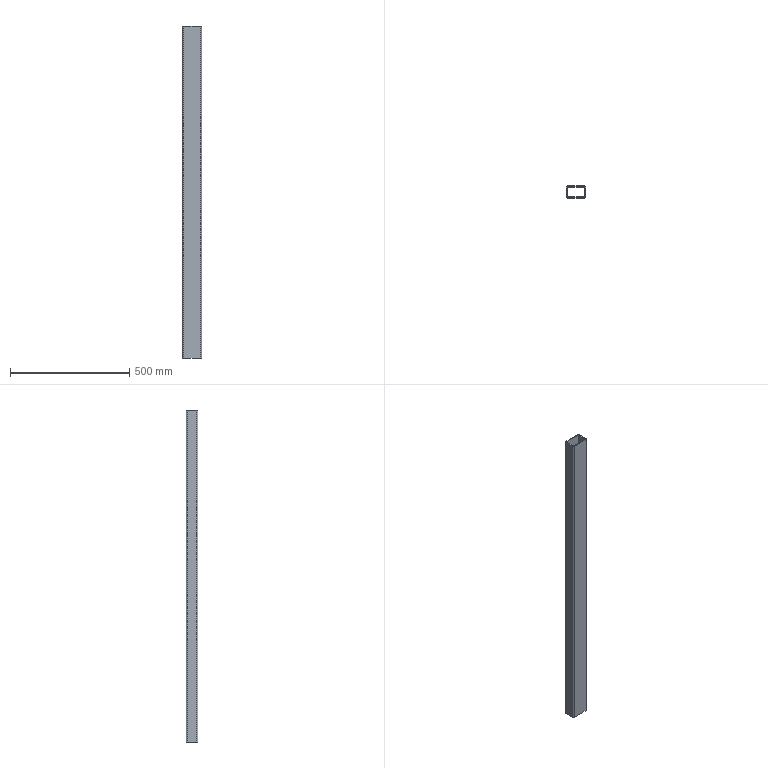Part | SolidWorks | features Extrusion 1, Shell 1 | 1 solid | 18 faces | box 80 x 50 x 1393 mm | volume 1330870 mm3 | plane 10 | cylinder 8 | commonest cylinder face diameters 2 x4 10 x4
STEP:
#1=CARTESIAN_POINT('',(-35.,25.,0.));
#2=VERTEX_POINT('',#1);
#3=CARTESIAN_POINT('',(-40.,20.,0.));
#4=VERTEX_POINT('',#3);
#5=CARTESIAN_POINT('',(-35.,20.,0.));
#6=DIRECTION('',(0.,0.,1.));
#7=DIRECTION('',(1.,0.,0.));
#8=AXIS2_PLACEMENT_3D('',#5,#6,#7);
#9=CIRCLE('',#8,5.);
#10=EDGE_CURVE('',#2,#4,#9,.T.);
#11=ORIENTED_EDGE('',*,*,#10,.T.);
#12=CARTESIAN_POINT('',(-40.,20.,1393.));
#13=VERTEX_POINT('',#12);
#14=CARTESIAN_POINT('',(-40.,20.,1393.));
#15=DIRECTION('',(0.,0.,-1.));
#16=VECTOR('',#15,1000.);
#17=LINE('',#14,#16);
#18=EDGE_CURVE('',#13,#4,#17,.T.);
#19=ORIENTED_EDGE('',*,*,#18,.F.);
#20=CARTESIAN_POINT('',(-35.,25.,1393.));
#21=VERTEX_POINT('',#20);
#22=CARTESIAN_POINT('',(-35.,20.,1393.));
#23=DIRECTION('',(0.,0.,1.));
#24=DIRECTION('',(1.,0.,0.));
#25=AXIS2_PLACEMENT_3D('',#22,#23,#24);
#26=CIRCLE('',#25,5.);
#27=EDGE_CURVE('',#21,#13,#26,.T.);
#28=ORIENTED_EDGE('',*,*,#27,.F.);
#29=CARTESIAN_POINT('',(-35.,25.,1393.));
#30=DIRECTION('',(0.,0.,-1.));
#31=VECTOR('',#30,1000.);
#32=LINE('',#29,#31);
#33=EDGE_CURVE('',#21,#2,#32,.T.);
#34=ORIENTED_EDGE('',*,*,#33,.T.);
#35=EDGE_LOOP('',(#11,#19,#28,#34));
#36=FACE_OUTER_BOUND('',#35,.T.);
#37=CARTESIAN_POINT('',(-35.,20.,1393.));
#38=DIRECTION('',(0.,0.,-1.));
#39=DIRECTION('',(-1.,0.,0.));
#40=AXIS2_PLACEMENT_3D('',#37,#38,#39);
#41=CYLINDRICAL_SURFACE('',#40,5.);
#42=ADVANCED_FACE('',(#36),#41,.T.);
#43=CARTESIAN_POINT('',(-40.,-20.,0.));
#44=VERTEX_POINT('',#43);
#45=CARTESIAN_POINT('',(-40.,20.,0.));
#46=DIRECTION('',(0.,-1.,0.));
#47=VECTOR('',#46,1000.);
#48=LINE('',#45,#47);
#49=EDGE_CURVE('',#4,#44,#48,.T.);
#50=ORIENTED_EDGE('',*,*,#49,.T.);
#51=CARTESIAN_POINT('',(-40.,-20.,1393.));
#52=VERTEX_POINT('',#51);
#53=CARTESIAN_POINT('',(-40.,-20.,1393.));
#54=DIRECTION('',(0.,0.,-1.));
#55=VECTOR('',#54,1000.);
#56=LINE('',#53,#55);
#57=EDGE_CURVE('',#52,#44,#56,.T.);
#58=ORIENTED_EDGE('',*,*,#57,.F.);
#59=CARTESIAN_POINT('',(-40.,20.,1393.));
#60=DIRECTION('',(0.,-1.,0.));
#61=VECTOR('',#60,1000.);
#62=LINE('',#59,#61);
#63=EDGE_CURVE('',#13,#52,#62,.T.);
#64=ORIENTED_EDGE('',*,*,#63,.F.);
#65=ORIENTED_EDGE('',*,*,#18,.T.);
#66=EDGE_LOOP('',(#50,#58,#64,#65));
#67=FACE_OUTER_BOUND('',#66,.T.);
#68=CARTESIAN_POINT('',(-40.,20.,1393.));
#69=DIRECTION('',(1.,0.,0.));
#70=DIRECTION('',(0.,0.,-1.));
#71=AXIS2_PLACEMENT_3D('',#68,#69,#70);
#72=PLANE('',#71);
#73=ADVANCED_FACE('',(#67),#72,.F.);
#74=CARTESIAN_POINT('',(-35.,-25.,0.));
#75=VERTEX_POINT('',#74);
#76=CARTESIAN_POINT('',(-35.,-20.,0.));
#77=DIRECTION('',(0.,0.,-1.));
#78=DIRECTION('',(-1.,0.,0.));
#79=AXIS2_PLACEMENT_3D('',#76,#77,#78);
#80=CIRCLE('',#79,5.);
#81=EDGE_CURVE('',#75,#44,#80,.T.);
#82=ORIENTED_EDGE('',*,*,#81,.F.);
#83=CARTESIAN_POINT('',(-35.,-25.,1393.));
#84=VERTEX_POINT('',#83);
#85=CARTESIAN_POINT('',(-35.,-25.,1393.));
#86=DIRECTION('',(0.,0.,-1.));
#87=VECTOR('',#86,1000.);
#88=LINE('',#85,#87);
#89=EDGE_CURVE('',#84,#75,#88,.T.);
#90=ORIENTED_EDGE('',*,*,#89,.F.);
#91=CARTESIAN_POINT('',(-35.,-20.,1393.));
#92=DIRECTION('',(0.,0.,-1.));
#93=DIRECTION('',(-1.,0.,0.));
#94=AXIS2_PLACEMENT_3D('',#91,#92,#93);
#95=CIRCLE('',#94,5.);
#96=EDGE_CURVE('',#84,#52,#95,.T.);
#97=ORIENTED_EDGE('',*,*,#96,.T.);
#98=ORIENTED_EDGE('',*,*,#57,.T.);
#99=EDGE_LOOP('',(#82,#90,#97,#98));
#100=FACE_OUTER_BOUND('',#99,.T.);
#101=CARTESIAN_POINT('',(-35.,-20.,1393.));
#102=DIRECTION('',(0.,0.,-1.));
#103=DIRECTION('',(-1.,0.,0.));
#104=AXIS2_PLACEMENT_3D('',#101,#102,#103);
#105=CYLINDRICAL_SURFACE('',#104,5.);
#106=ADVANCED_FACE('',(#100),#105,.T.);
#107=CARTESIAN_POINT('',(35.,-25.,0.));
#108=VERTEX_POINT('',#107);
#109=CARTESIAN_POINT('',(35.,-25.,0.));
#110=DIRECTION('',(-1.,0.,0.));
#111=VECTOR('',#110,1000.);
#112=LINE('',#109,#111);
#113=EDGE_CURVE('',#108,#75,#112,.T.);
#114=ORIENTED_EDGE('',*,*,#113,.F.);
#115=CARTESIAN_POINT('',(35.,-25.,1393.));
#116=VERTEX_POINT('',#115);
#117=CARTESIAN_POINT('',(35.,-25.,1393.));
#118=DIRECTION('',(0.,0.,-1.));
#119=VECTOR('',#118,1000.);
#120=LINE('',#117,#119);
#121=EDGE_CURVE('',#116,#108,#120,.T.);
#122=ORIENTED_EDGE('',*,*,#121,.F.);
#123=CARTESIAN_POINT('',(35.,-25.,1393.));
#124=DIRECTION('',(-1.,0.,0.));
#125=VECTOR('',#124,1000.);
#126=LINE('',#123,#125);
#127=EDGE_CURVE('',#116,#84,#126,.T.);
#128=ORIENTED_EDGE('',*,*,#127,.T.);
#129=ORIENTED_EDGE('',*,*,#89,.T.);
#130=EDGE_LOOP('',(#114,#122,#128,#129));
#131=FACE_OUTER_BOUND('',#130,.T.);
#132=CARTESIAN_POINT('',(35.,-25.,1393.));
#133=DIRECTION('',(0.,-1.,0.));
#134=DIRECTION('',(1.,0.,0.));
#135=AXIS2_PLACEMENT_3D('',#132,#133,#134);
#136=PLANE('',#135);
#137=ADVANCED_FACE('',(#131),#136,.T.);
#138=CARTESIAN_POINT('',(40.,-20.,0.));
#139=VERTEX_POINT('',#138);
#140=CARTESIAN_POINT('',(35.,-20.,0.));
#141=DIRECTION('',(0.,0.,-1.));
#142=DIRECTION('',(-1.,0.,0.));
#143=AXIS2_PLACEMENT_3D('',#140,#141,#142);
#144=CIRCLE('',#143,5.);
#145=EDGE_CURVE('',#139,#108,#144,.T.);
#146=ORIENTED_EDGE('',*,*,#145,.F.);
#147=CARTESIAN_POINT('',(40.,-20.,1393.));
#148=VERTEX_POINT('',#147);
#149=CARTESIAN_POINT('',(40.,-20.,1393.));
#150=DIRECTION('',(0.,0.,-1.));
#151=VECTOR('',#150,1000.);
#152=LINE('',#149,#151);
#153=EDGE_CURVE('',#148,#139,#152,.T.);
#154=ORIENTED_EDGE('',*,*,#153,.F.);
#155=CARTESIAN_POINT('',(35.,-20.,1393.));
#156=DIRECTION('',(0.,0.,-1.));
#157=DIRECTION('',(-1.,0.,0.));
#158=AXIS2_PLACEMENT_3D('',#155,#156,#157);
#159=CIRCLE('',#158,5.);
#160=EDGE_CURVE('',#148,#116,#159,.T.);
#161=ORIENTED_EDGE('',*,*,#160,.T.);
#162=ORIENTED_EDGE('',*,*,#121,.T.);
#163=EDGE_LOOP('',(#146,#154,#161,#162));
#164=FACE_OUTER_BOUND('',#163,.T.);
#165=CARTESIAN_POINT('',(35.,-20.,1393.));
#166=DIRECTION('',(0.,0.,-1.));
#167=DIRECTION('',(-1.,0.,0.));
#168=AXIS2_PLACEMENT_3D('',#165,#166,#167);
#169=CYLINDRICAL_SURFACE('',#168,5.);
#170=ADVANCED_FACE('',(#164),#169,.T.);
#171=CARTESIAN_POINT('',(40.,20.,0.));
#172=VERTEX_POINT('',#171);
#173=CARTESIAN_POINT('',(40.,20.,0.));
#174=DIRECTION('',(0.,-1.,0.));
#175=VECTOR('',#174,1000.);
#176=LINE('',#173,#175);
#177=EDGE_CURVE('',#172,#139,#176,.T.);
#178=ORIENTED_EDGE('',*,*,#177,.F.);
#179=CARTESIAN_POINT('',(40.,20.,1393.));
#180=VERTEX_POINT('',#179);
#181=CARTESIAN_POINT('',(40.,20.,1393.));
#182=DIRECTION('',(0.,0.,-1.));
#183=VECTOR('',#182,1000.);
#184=LINE('',#181,#183);
#185=EDGE_CURVE('',#180,#172,#184,.T.);
#186=ORIENTED_EDGE('',*,*,#185,.F.);
#187=CARTESIAN_POINT('',(40.,20.,1393.));
#188=DIRECTION('',(0.,-1.,0.));
#189=VECTOR('',#188,1000.);
#190=LINE('',#187,#189);
#191=EDGE_CURVE('',#180,#148,#190,.T.);
#192=ORIENTED_EDGE('',*,*,#191,.T.);
#193=ORIENTED_EDGE('',*,*,#153,.T.);
#194=EDGE_LOOP('',(#178,#186,#192,#193));
#195=FACE_OUTER_BOUND('',#194,.T.);
#196=CARTESIAN_POINT('',(40.,20.,1393.));
#197=DIRECTION('',(1.,0.,0.));
#198=DIRECTION('',(0.,1.,0.));
#199=AXIS2_PLACEMENT_3D('',#196,#197,#198);
#200=PLANE('',#199);
#201=ADVANCED_FACE('',(#195),#200,.T.);
#202=CARTESIAN_POINT('',(35.,25.,0.));
#203=VERTEX_POINT('',#202);
#204=CARTESIAN_POINT('',(35.,20.,0.));
#205=DIRECTION('',(0.,0.,-1.));
#206=DIRECTION('',(-1.,0.,0.));
#207=AXIS2_PLACEMENT_3D('',#204,#205,#206);
#208=CIRCLE('',#207,5.);
#209=EDGE_CURVE('',#203,#172,#208,.T.);
#210=ORIENTED_EDGE('',*,*,#209,.F.);
#211=CARTESIAN_POINT('',(35.,25.,1393.));
#212=VERTEX_POINT('',#211);
#213=CARTESIAN_POINT('',(35.,25.,1393.));
#214=DIRECTION('',(0.,0.,-1.));
#215=VECTOR('',#214,1000.);
#216=LINE('',#213,#215);
#217=EDGE_CURVE('',#212,#203,#216,.T.);
#218=ORIENTED_EDGE('',*,*,#217,.F.);
#219=CARTESIAN_POINT('',(35.,20.,1393.));
#220=DIRECTION('',(0.,0.,-1.));
#221=DIRECTION('',(-1.,0.,0.));
#222=AXIS2_PLACEMENT_3D('',#219,#220,#221);
#223=CIRCLE('',#222,5.);
#224=EDGE_CURVE('',#212,#180,#223,.T.);
#225=ORIENTED_EDGE('',*,*,#224,.T.);
#226=ORIENTED_EDGE('',*,*,#185,.T.);
#227=EDGE_LOOP('',(#210,#218,#225,#226));
#228=FACE_OUTER_BOUND('',#227,.T.);
#229=CARTESIAN_POINT('',(35.,20.,1393.));
#230=DIRECTION('',(0.,0.,-1.));
#231=DIRECTION('',(-1.,0.,0.));
#232=AXIS2_PLACEMENT_3D('',#229,#230,#231);
#233=CYLINDRICAL_SURFACE('',#232,5.);
#234=ADVANCED_FACE('',(#228),#233,.T.);
#235=CARTESIAN_POINT('',(35.,25.,0.));
#236=DIRECTION('',(-1.,0.,0.));
#237=VECTOR('',#236,1000.);
#238=LINE('',#235,#237);
#239=EDGE_CURVE('',#203,#2,#238,.T.);
#240=ORIENTED_EDGE('',*,*,#239,.T.);
#241=ORIENTED_EDGE('',*,*,#33,.F.);
#242=CARTESIAN_POINT('',(35.,25.,1393.));
#243=DIRECTION('',(-1.,0.,0.));
#244=VECTOR('',#243,1000.);
#245=LINE('',#242,#244);
#246=EDGE_CURVE('',#212,#21,#245,.T.);
#247=ORIENTED_EDGE('',*,*,#246,.F.);
#248=ORIENTED_EDGE('',*,*,#217,.T.);
#249=EDGE_LOOP('',(#240,#241,#247,#248));
#250=FACE_OUTER_BOUND('',#249,.T.);
#251=CARTESIAN_POINT('',(35.,25.,1393.));
#252=DIRECTION('',(0.,-1.,0.));
#253=DIRECTION('',(1.,0.,0.));
#254=AXIS2_PLACEMENT_3D('',#251,#252,#253);
#255=PLANE('',#254);
#256=ADVANCED_FACE('',(#250),#255,.F.);
#257=CARTESIAN_POINT('',(-35.,21.,1393.));
#258=VERTEX_POINT('',#257);
#259=CARTESIAN_POINT('',(-36.,20.,1393.));
#260=VERTEX_POINT('',#259);
#261=CARTESIAN_POINT('',(-35.,20.,1393.));
#262=DIRECTION('',(0.,0.,1.));
#263=DIRECTION('',(1.,0.,0.));
#264=AXIS2_PLACEMENT_3D('',#261,#262,#263);
#265=CIRCLE('',#264,1.);
#266=EDGE_CURVE('',#258,#260,#265,.T.);
#267=ORIENTED_EDGE('',*,*,#266,.F.);
#268=CARTESIAN_POINT('',(35.,21.,1393.));
#269=VERTEX_POINT('',#268);
#270=CARTESIAN_POINT('',(35.,21.,1393.));
#271=DIRECTION('',(-1.,0.,0.));
#272=VECTOR('',#271,1000.);
#273=LINE('',#270,#272);
#274=EDGE_CURVE('',#269,#258,#273,.T.);
#275=ORIENTED_EDGE('',*,*,#274,.F.);
#276=CARTESIAN_POINT('',(36.,20.,1393.));
#277=VERTEX_POINT('',#276);
#278=CARTESIAN_POINT('',(35.,20.,1393.));
#279=DIRECTION('',(0.,0.,-1.));
#280=DIRECTION('',(1.,0.,0.));
#281=AXIS2_PLACEMENT_3D('',#278,#279,#280);
#282=CIRCLE('',#281,1.);
#283=EDGE_CURVE('',#269,#277,#282,.T.);
#284=ORIENTED_EDGE('',*,*,#283,.T.);
#285=CARTESIAN_POINT('',(36.,-20.,1393.));
#286=VERTEX_POINT('',#285);
#287=CARTESIAN_POINT('',(36.,20.,1393.));
#288=DIRECTION('',(0.,-1.,0.));
#289=VECTOR('',#288,1000.);
#290=LINE('',#287,#289);
#291=EDGE_CURVE('',#277,#286,#290,.T.);
#292=ORIENTED_EDGE('',*,*,#291,.T.);
#293=CARTESIAN_POINT('',(35.,-21.,1393.));
#294=VERTEX_POINT('',#293);
#295=CARTESIAN_POINT('',(35.,-20.,1393.));
#296=DIRECTION('',(0.,0.,-1.));
#297=DIRECTION('',(1.,0.,0.));
#298=AXIS2_PLACEMENT_3D('',#295,#296,#297);
#299=CIRCLE('',#298,1.);
#300=EDGE_CURVE('',#286,#294,#299,.T.);
#301=ORIENTED_EDGE('',*,*,#300,.T.);
#302=CARTESIAN_POINT('',(-35.,-21.,1393.));
#303=VERTEX_POINT('',#302);
#304=CARTESIAN_POINT('',(35.,-21.,1393.));
#305=DIRECTION('',(-1.,0.,0.));
#306=VECTOR('',#305,1000.);
#307=LINE('',#304,#306);
#308=EDGE_CURVE('',#294,#303,#307,.T.);
#309=ORIENTED_EDGE('',*,*,#308,.T.);
#310=CARTESIAN_POINT('',(-36.,-20.,1393.));
#311=VERTEX_POINT('',#310);
#312=CARTESIAN_POINT('',(-35.,-20.,1393.));
#313=DIRECTION('',(0.,0.,-1.));
#314=DIRECTION('',(1.,0.,0.));
#315=AXIS2_PLACEMENT_3D('',#312,#313,#314);
#316=CIRCLE('',#315,1.);
#317=EDGE_CURVE('',#303,#311,#316,.T.);
#318=ORIENTED_EDGE('',*,*,#317,.T.);
#319=CARTESIAN_POINT('',(-36.,20.,1393.));
#320=DIRECTION('',(0.,-1.,0.));
#321=VECTOR('',#320,1000.);
#322=LINE('',#319,#321);
#323=EDGE_CURVE('',#260,#311,#322,.T.);
#324=ORIENTED_EDGE('',*,*,#323,.F.);
#325=EDGE_LOOP('',(#267,#275,#284,#292,#301,#309,#318,#324));
#326=FACE_BOUND('',#325,.T.);
#327=ORIENTED_EDGE('',*,*,#27,.T.);
#328=ORIENTED_EDGE('',*,*,#63,.T.);
#329=ORIENTED_EDGE('',*,*,#96,.F.);
#330=ORIENTED_EDGE('',*,*,#127,.F.);
#331=ORIENTED_EDGE('',*,*,#160,.F.);
#332=ORIENTED_EDGE('',*,*,#191,.F.);
#333=ORIENTED_EDGE('',*,*,#224,.F.);
#334=ORIENTED_EDGE('',*,*,#246,.T.);
#335=EDGE_LOOP('',(#327,#328,#329,#330,#331,#332,#333,#334));
#336=FACE_OUTER_BOUND('',#335,.T.);
#337=CARTESIAN_POINT('',(-35.,20.,1393.));
#338=DIRECTION('',(0.,0.,1.));
#339=DIRECTION('',(1.,0.,0.));
#340=AXIS2_PLACEMENT_3D('',#337,#338,#339);
#341=PLANE('',#340);
#342=ADVANCED_FACE('',(#326,#336),#341,.T.);
#343=CARTESIAN_POINT('',(35.,21.,0.));
#344=VERTEX_POINT('',#343);
#345=CARTESIAN_POINT('',(-35.,21.,0.));
#346=VERTEX_POINT('',#345);
#347=CARTESIAN_POINT('',(35.,21.,0.));
#348=DIRECTION('',(-1.,0.,0.));
#349=VECTOR('',#348,1000.);
#350=LINE('',#347,#349);
#351=EDGE_CURVE('',#344,#346,#350,.T.);
#352=ORIENTED_EDGE('',*,*,#351,.T.);
#353=CARTESIAN_POINT('',(-36.,20.,0.));
#354=VERTEX_POINT('',#353);
#355=CARTESIAN_POINT('',(-35.,20.,0.));
#356=DIRECTION('',(0.,0.,1.));
#357=DIRECTION('',(1.,0.,0.));
#358=AXIS2_PLACEMENT_3D('',#355,#356,#357);
#359=CIRCLE('',#358,1.);
#360=EDGE_CURVE('',#346,#354,#359,.T.);
#361=ORIENTED_EDGE('',*,*,#360,.T.);
#362=CARTESIAN_POINT('',(-36.,-20.,0.));
#363=VERTEX_POINT('',#362);
#364=CARTESIAN_POINT('',(-36.,20.,0.));
#365=DIRECTION('',(0.,-1.,0.));
#366=VECTOR('',#365,1000.);
#367=LINE('',#364,#366);
#368=EDGE_CURVE('',#354,#363,#367,.T.);
#369=ORIENTED_EDGE('',*,*,#368,.T.);
#370=CARTESIAN_POINT('',(-35.,-21.,0.));
#371=VERTEX_POINT('',#370);
#372=CARTESIAN_POINT('',(-35.,-20.,0.));
#373=DIRECTION('',(0.,0.,-1.));
#374=DIRECTION('',(1.,0.,0.));
#375=AXIS2_PLACEMENT_3D('',#372,#373,#374);
#376=CIRCLE('',#375,1.);
#377=EDGE_CURVE('',#371,#363,#376,.T.);
#378=ORIENTED_EDGE('',*,*,#377,.F.);
#379=CARTESIAN_POINT('',(35.,-21.,0.));
#380=VERTEX_POINT('',#379);
#381=CARTESIAN_POINT('',(35.,-21.,0.));
#382=DIRECTION('',(-1.,0.,0.));
#383=VECTOR('',#382,1000.);
#384=LINE('',#381,#383);
#385=EDGE_CURVE('',#380,#371,#384,.T.);
#386=ORIENTED_EDGE('',*,*,#385,.F.);
#387=CARTESIAN_POINT('',(36.,-20.,0.));
#388=VERTEX_POINT('',#387);
#389=CARTESIAN_POINT('',(35.,-20.,0.));
#390=DIRECTION('',(0.,0.,-1.));
#391=DIRECTION('',(1.,0.,0.));
#392=AXIS2_PLACEMENT_3D('',#389,#390,#391);
#393=CIRCLE('',#392,1.);
#394=EDGE_CURVE('',#388,#380,#393,.T.);
#395=ORIENTED_EDGE('',*,*,#394,.F.);
#396=CARTESIAN_POINT('',(36.,20.,0.));
#397=VERTEX_POINT('',#396);
#398=CARTESIAN_POINT('',(36.,20.,0.));
#399=DIRECTION('',(0.,-1.,0.));
#400=VECTOR('',#399,1000.);
#401=LINE('',#398,#400);
#402=EDGE_CURVE('',#397,#388,#401,.T.);
#403=ORIENTED_EDGE('',*,*,#402,.F.);
#404=CARTESIAN_POINT('',(35.,20.,0.));
#405=DIRECTION('',(0.,0.,-1.));
#406=DIRECTION('',(1.,0.,0.));
#407=AXIS2_PLACEMENT_3D('',#404,#405,#406);
#408=CIRCLE('',#407,1.);
#409=EDGE_CURVE('',#344,#397,#408,.T.);
#410=ORIENTED_EDGE('',*,*,#409,.F.);
#411=EDGE_LOOP('',(#352,#361,#369,#378,#386,#395,#403,#410));
#412=FACE_BOUND('',#411,.T.);
#413=ORIENTED_EDGE('',*,*,#10,.F.);
#414=ORIENTED_EDGE('',*,*,#239,.F.);
#415=ORIENTED_EDGE('',*,*,#209,.T.);
#416=ORIENTED_EDGE('',*,*,#177,.T.);
#417=ORIENTED_EDGE('',*,*,#145,.T.);
#418=ORIENTED_EDGE('',*,*,#113,.T.);
#419=ORIENTED_EDGE('',*,*,#81,.T.);
#420=ORIENTED_EDGE('',*,*,#49,.F.);
#421=EDGE_LOOP('',(#413,#414,#415,#416,#417,#418,#419,#420));
#422=FACE_OUTER_BOUND('',#421,.T.);
#423=CARTESIAN_POINT('',(-35.,20.,0.));
#424=DIRECTION('',(0.,0.,1.));
#425=DIRECTION('',(1.,0.,0.));
#426=AXIS2_PLACEMENT_3D('',#423,#424,#425);
#427=PLANE('',#426);
#428=ADVANCED_FACE('',(#412,#422),#427,.F.);
#429=ORIENTED_EDGE('',*,*,#360,.F.);
#430=CARTESIAN_POINT('',(-35.,21.,1393.));
#431=DIRECTION('',(0.,0.,-1.));
#432=VECTOR('',#431,1000.);
#433=LINE('',#430,#432);
#434=EDGE_CURVE('',#258,#346,#433,.T.);
#435=ORIENTED_EDGE('',*,*,#434,.F.);
#436=ORIENTED_EDGE('',*,*,#266,.T.);
#437=CARTESIAN_POINT('',(-36.,20.,1393.));
#438=DIRECTION('',(0.,0.,-1.));
#439=VECTOR('',#438,1000.);
#440=LINE('',#437,#439);
#441=EDGE_CURVE('',#260,#354,#440,.T.);
#442=ORIENTED_EDGE('',*,*,#441,.T.);
#443=EDGE_LOOP('',(#429,#435,#436,#442));
#444=FACE_OUTER_BOUND('',#443,.T.);
#445=CARTESIAN_POINT('',(-35.,20.,1393.));
#446=DIRECTION('',(0.,0.,-1.));
#447=DIRECTION('',(-1.,0.,0.));
#448=AXIS2_PLACEMENT_3D('',#445,#446,#447);
#449=CYLINDRICAL_SURFACE('',#448,1.);
#450=ADVANCED_FACE('',(#444),#449,.F.);
#451=ORIENTED_EDGE('',*,*,#368,.F.);
#452=ORIENTED_EDGE('',*,*,#441,.F.);
#453=ORIENTED_EDGE('',*,*,#323,.T.);
#454=CARTESIAN_POINT('',(-36.,-20.,1393.));
#455=DIRECTION('',(0.,0.,-1.));
#456=VECTOR('',#455,1000.);
#457=LINE('',#454,#456);
#458=EDGE_CURVE('',#311,#363,#457,.T.);
#459=ORIENTED_EDGE('',*,*,#458,.T.);
#460=EDGE_LOOP('',(#451,#452,#453,#459));
#461=FACE_OUTER_BOUND('',#460,.T.);
#462=CARTESIAN_POINT('',(-36.,20.,1393.));
#463=DIRECTION('',(1.,0.,0.));
#464=DIRECTION('',(0.,0.,-1.));
#465=AXIS2_PLACEMENT_3D('',#462,#463,#464);
#466=PLANE('',#465);
#467=ADVANCED_FACE('',(#461),#466,.T.);
#468=ORIENTED_EDGE('',*,*,#377,.T.);
#469=ORIENTED_EDGE('',*,*,#458,.F.);
#470=ORIENTED_EDGE('',*,*,#317,.F.);
#471=CARTESIAN_POINT('',(-35.,-21.,1393.));
#472=DIRECTION('',(0.,0.,-1.));
#473=VECTOR('',#472,1000.);
#474=LINE('',#471,#473);
#475=EDGE_CURVE('',#303,#371,#474,.T.);
#476=ORIENTED_EDGE('',*,*,#475,.T.);
#477=EDGE_LOOP('',(#468,#469,#470,#476));
#478=FACE_OUTER_BOUND('',#477,.T.);
#479=CARTESIAN_POINT('',(-35.,-20.,1393.));
#480=DIRECTION('',(0.,0.,-1.));
#481=DIRECTION('',(-1.,0.,0.));
#482=AXIS2_PLACEMENT_3D('',#479,#480,#481);
#483=CYLINDRICAL_SURFACE('',#482,1.);
#484=ADVANCED_FACE('',(#478),#483,.F.);
#485=ORIENTED_EDGE('',*,*,#385,.T.);
#486=ORIENTED_EDGE('',*,*,#475,.F.);
#487=ORIENTED_EDGE('',*,*,#308,.F.);
#488=CARTESIAN_POINT('',(35.,-21.,1393.));
#489=DIRECTION('',(0.,0.,-1.));
#490=VECTOR('',#489,1000.);
#491=LINE('',#488,#490);
#492=EDGE_CURVE('',#294,#380,#491,.T.);
#493=ORIENTED_EDGE('',*,*,#492,.T.);
#494=EDGE_LOOP('',(#485,#486,#487,#493));
#495=FACE_OUTER_BOUND('',#494,.T.);
#496=CARTESIAN_POINT('',(35.,-21.,1393.));
#497=DIRECTION('',(0.,-1.,0.));
#498=DIRECTION('',(1.,0.,0.));
#499=AXIS2_PLACEMENT_3D('',#496,#497,#498);
#500=PLANE('',#499);
#501=ADVANCED_FACE('',(#495),#500,.F.);
#502=ORIENTED_EDGE('',*,*,#394,.T.);
#503=ORIENTED_EDGE('',*,*,#492,.F.);
#504=ORIENTED_EDGE('',*,*,#300,.F.);
#505=CARTESIAN_POINT('',(36.,-20.,1393.));
#506=DIRECTION('',(0.,0.,-1.));
#507=VECTOR('',#506,1000.);
#508=LINE('',#505,#507);
#509=EDGE_CURVE('',#286,#388,#508,.T.);
#510=ORIENTED_EDGE('',*,*,#509,.T.);
#511=EDGE_LOOP('',(#502,#503,#504,#510));
#512=FACE_OUTER_BOUND('',#511,.T.);
#513=CARTESIAN_POINT('',(35.,-20.,1393.));
#514=DIRECTION('',(0.,0.,-1.));
#515=DIRECTION('',(-1.,0.,0.));
#516=AXIS2_PLACEMENT_3D('',#513,#514,#515);
#517=CYLINDRICAL_SURFACE('',#516,1.);
#518=ADVANCED_FACE('',(#512),#517,.F.);
#519=ORIENTED_EDGE('',*,*,#402,.T.);
#520=ORIENTED_EDGE('',*,*,#509,.F.);
#521=ORIENTED_EDGE('',*,*,#291,.F.);
#522=CARTESIAN_POINT('',(36.,20.,1393.));
#523=DIRECTION('',(0.,0.,-1.));
#524=VECTOR('',#523,1000.);
#525=LINE('',#522,#524);
#526=EDGE_CURVE('',#277,#397,#525,.T.);
#527=ORIENTED_EDGE('',*,*,#526,.T.);
#528=EDGE_LOOP('',(#519,#520,#521,#527));
#529=FACE_OUTER_BOUND('',#528,.T.);
#530=CARTESIAN_POINT('',(36.,20.,1393.));
#531=DIRECTION('',(1.,0.,0.));
#532=DIRECTION('',(0.,1.,0.));
#533=AXIS2_PLACEMENT_3D('',#530,#531,#532);
#534=PLANE('',#533);
#535=ADVANCED_FACE('',(#529),#534,.F.);
#536=ORIENTED_EDGE('',*,*,#409,.T.);
#537=ORIENTED_EDGE('',*,*,#526,.F.);
#538=ORIENTED_EDGE('',*,*,#283,.F.);
#539=CARTESIAN_POINT('',(35.,21.,1393.));
#540=DIRECTION('',(0.,0.,-1.));
#541=VECTOR('',#540,1000.);
#542=LINE('',#539,#541);
#543=EDGE_CURVE('',#269,#344,#542,.T.);
#544=ORIENTED_EDGE('',*,*,#543,.T.);
#545=EDGE_LOOP('',(#536,#537,#538,#544));
#546=FACE_OUTER_BOUND('',#545,.T.);
#547=CARTESIAN_POINT('',(35.,20.,1393.));
#548=DIRECTION('',(0.,0.,-1.));
#549=DIRECTION('',(-1.,0.,0.));
#550=AXIS2_PLACEMENT_3D('',#547,#548,#549);
#551=CYLINDRICAL_SURFACE('',#550,1.);
#552=ADVANCED_FACE('',(#546),#551,.F.);
#553=ORIENTED_EDGE('',*,*,#351,.F.);
#554=ORIENTED_EDGE('',*,*,#543,.F.);
#555=ORIENTED_EDGE('',*,*,#274,.T.);
#556=ORIENTED_EDGE('',*,*,#434,.T.);
#557=EDGE_LOOP('',(#553,#554,#555,#556));
#558=FACE_OUTER_BOUND('',#557,.T.);
#559=CARTESIAN_POINT('',(35.,21.,1393.));
#560=DIRECTION('',(0.,-1.,0.));
#561=DIRECTION('',(1.,0.,0.));
#562=AXIS2_PLACEMENT_3D('',#559,#560,#561);
#563=PLANE('',#562);
#564=ADVANCED_FACE('',(#558),#563,.T.);
#565=CLOSED_SHELL('',(#42,#73,#106,#137,#170,#201,#234,#256,#342,#428,#450,#467,#484,#501,#518,#535,#552,#564));
#566=MANIFOLD_SOLID_BREP('',#565);
#567=CARTESIAN_POINT('',(0.,0.,0.));
#568=DIRECTION('',(0.,0.,1.));
#569=DIRECTION('',(1.,0.,0.));
#570=AXIS2_PLACEMENT_3D('',#567,#568,#569);
#571=(LENGTH_UNIT()NAMED_UNIT(*)SI_UNIT(.MILLI.,.METRE.));
#572=UNCERTAINTY_MEASURE_WITH_UNIT(LENGTH_MEASURE(0.00001),#571,'','');
#573=(NAMED_UNIT(*)PLANE_ANGLE_UNIT()SI_UNIT($,.RADIAN.));
#574=(NAMED_UNIT(*)SI_UNIT($,.STERADIAN.)SOLID_ANGLE_UNIT());
#575=(GEOMETRIC_REPRESENTATION_CONTEXT(3)GLOBAL_UNCERTAINTY_ASSIGNED_CONTEXT((#572))GLOBAL_UNIT_ASSIGNED_CONTEXT((#571,#573,#574))REPRESENTATION_CONTEXT('',''));
#576=ADVANCED_BREP_SHAPE_REPRESENTATION('',(#566,#570),#575);